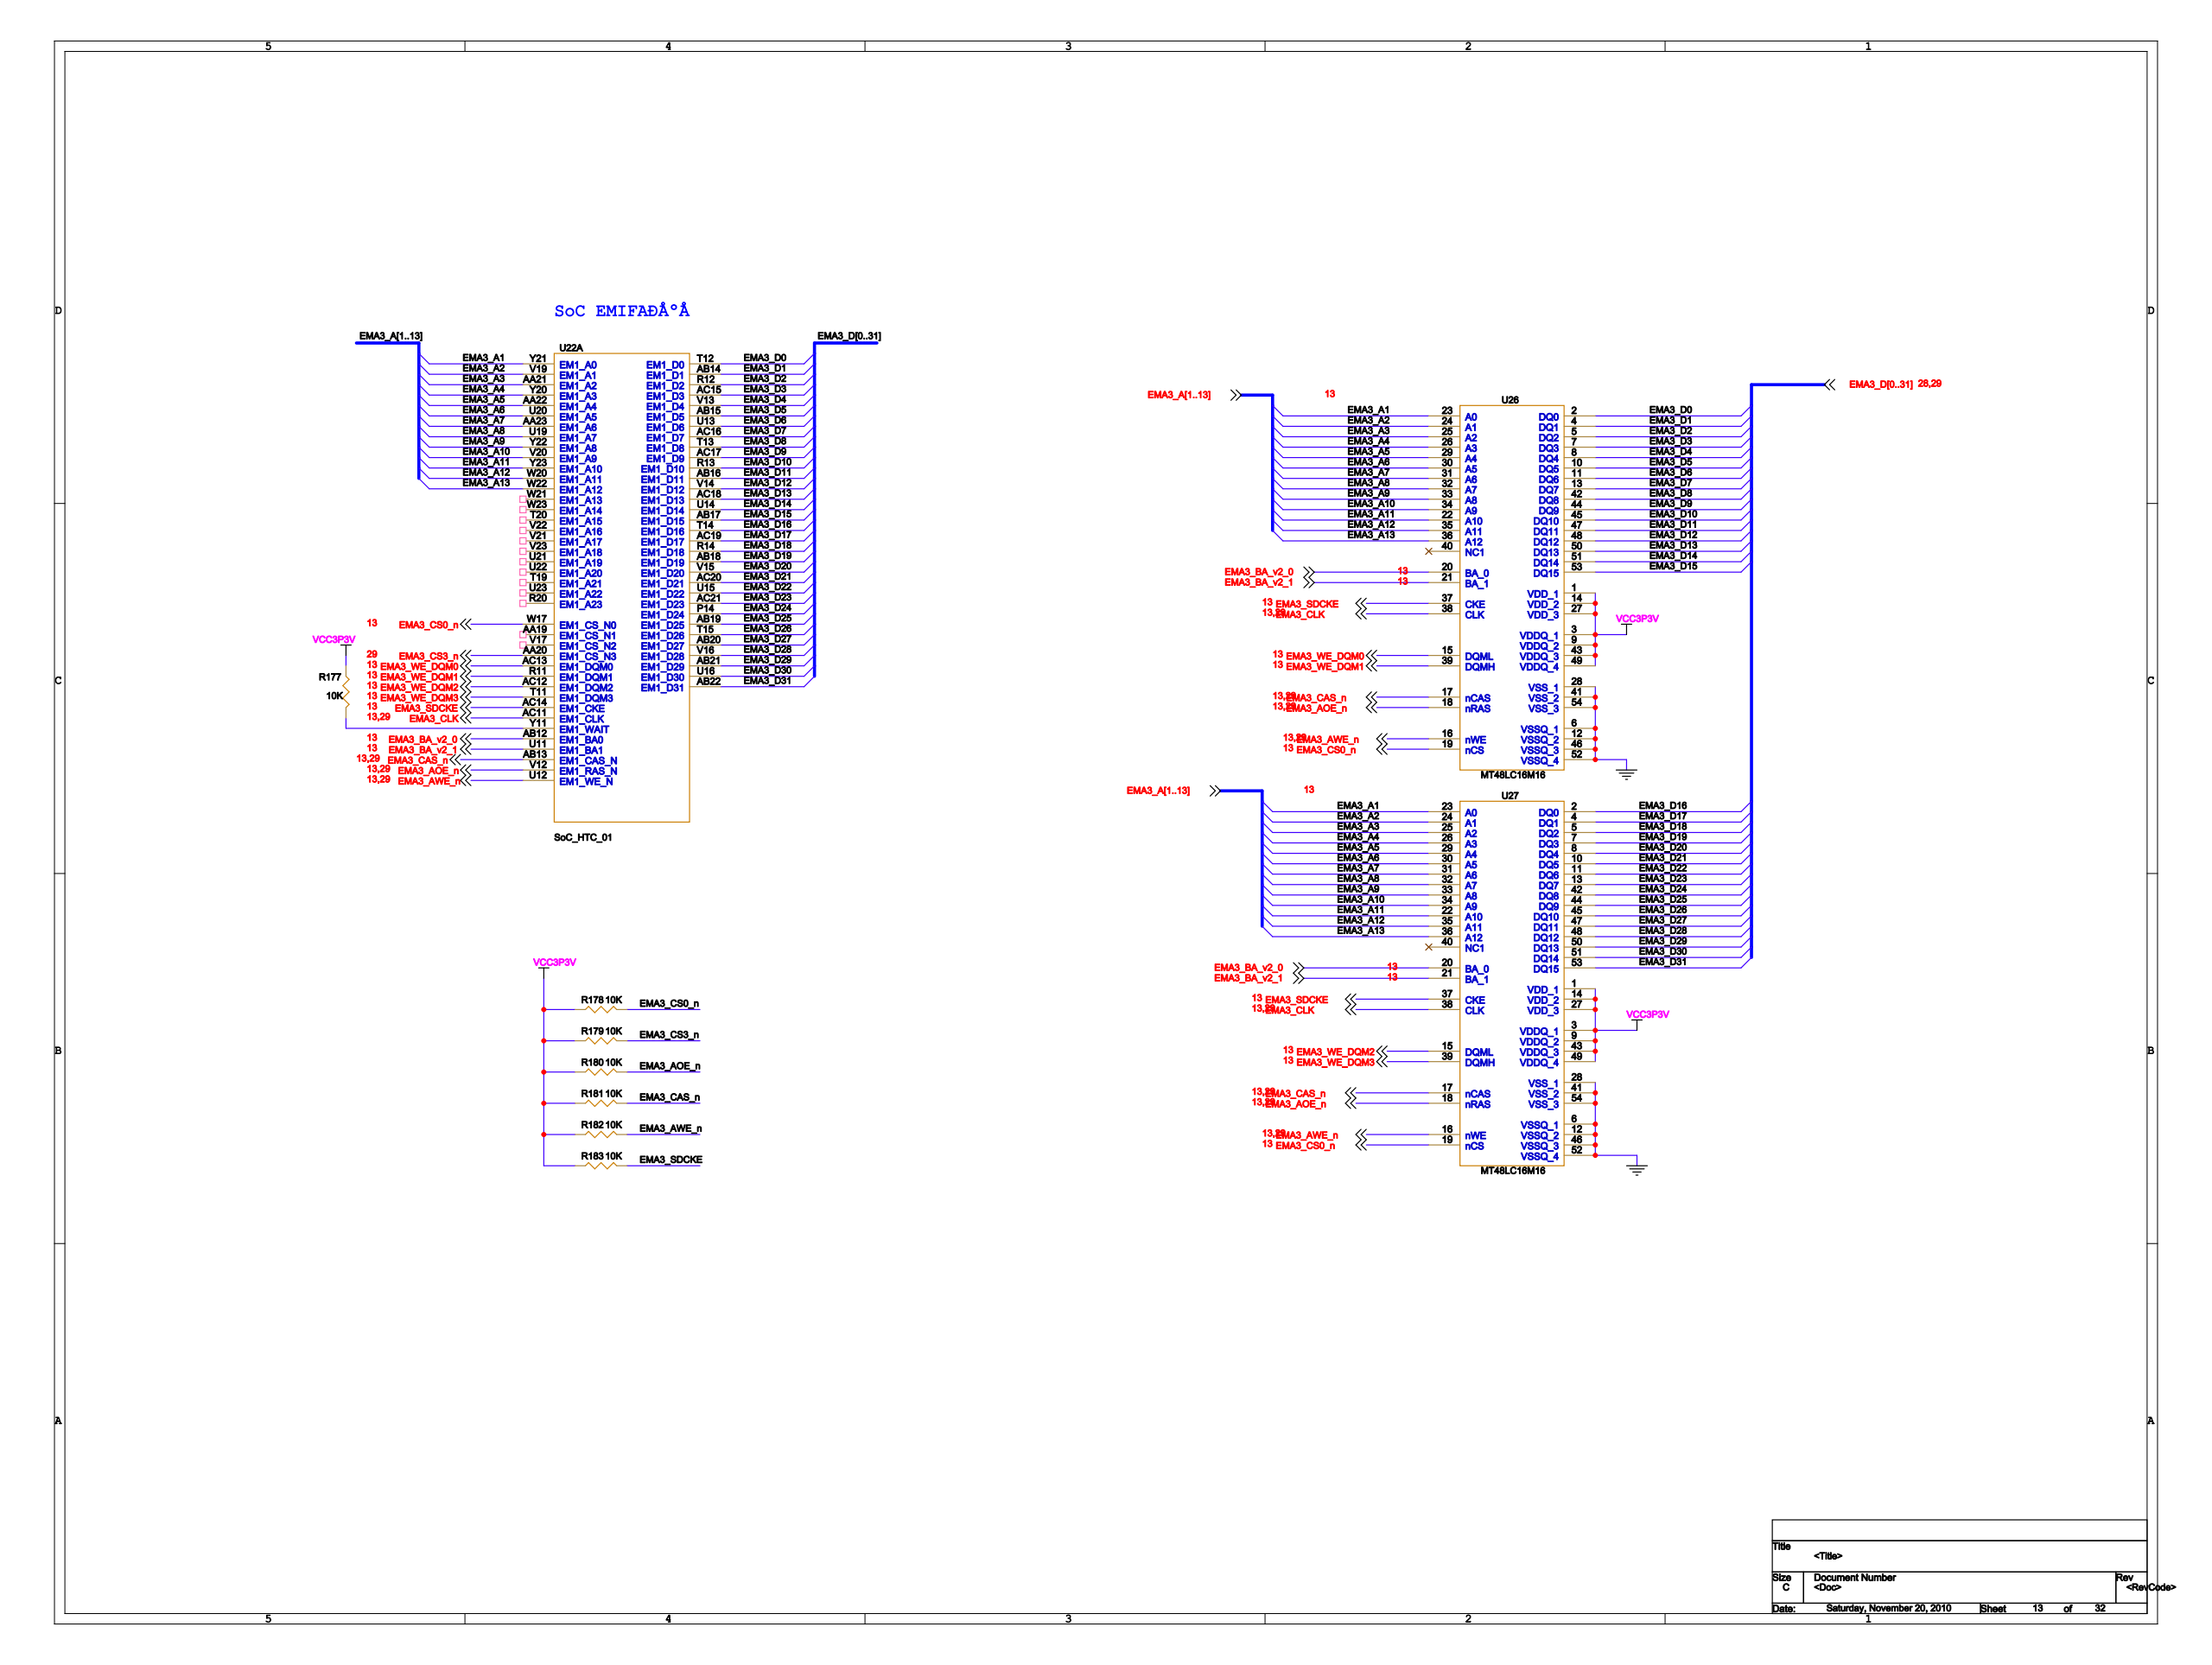Circuit board | Cadence Allegro | 1001 parts | 1318 nets | one sheet of the schematic
Parts on this sheet (reference | value | footprint):
R177 | 10K | 0603
R178 | 10K | 0603
R179 | 10K | 0603
R180 | 10K | 0603
R181 | 10K | 0603
R182 | 10K | 0603
R183 | 10K | 0603
U11 | MT48LC32M16 | TSOP54
U14 | MT48LC16M16 | TSOP54
U15 | MT48LC16M16 | TSOP54
U20 | MT48LC16M16 | TSOP54
U21 | MT48LC16M16 | TSOP54
U22 | SoC_HTC_01 | L529_XIN
U23 | MT48LC32M16 | TSOP54
U26 | MT48LC16M16 | TSOP54
U27 | MT48LC16M16 | TSOP54
Nets of these parts (net: part-pin ...):
EMA3_AWE_N: R182-2 U22-U12 U26-16 U27-16
EMA3_D6: U22-U13 U26-11
EMA3_D0: U22-T12 U26-2
EMA3_D2: U22-R12 U26-5
EMA3_D8: U22-T13 U26-42
EMA3_D10: U22-R13 U26-45
EMA3_D18: U22-R14 U27-5
EMA3_CLK: U22-AC11 U26-38 U27-38
EMA3_D16: U22-T14 U27-2
EMA3_D24: U22-P14 U27-42
EMA3_D22: U22-U15 U27-11
EMA3_D20: U22-V15 U27-8
EMA3_D26: U22-T15 U27-45
EMA3_D30: U22-U16 U27-51
EMA3_D23: U22-AC21 U27-13
EMA3_D31: U22-AB22 U27-53
EMA3_D14: U22-U14 U26-51
EMA3_D12: U22-V14 U26-48
EMA3_D28: U22-V16 U27-48
EMA3_CAS_N: R181-2 U22-AB13 U26-17 U27-17
EMA3_D5: U22-AB15 U26-10
EMA3_D1: U22-AB14 U26-4
EMA3_D3: U22-AC15 U26-7
EMA3_D11: U22-AB16 U26-47
EMA3_D15: U22-AB17 U26-53
EMA3_D7: U22-AC16 U26-13
EMA3_D25: U22-AB19 U27-44
EMA3_D19: U22-AB18 U27-7
EMA3_D9: U22-AC17 U26-44
EMA3_D21: U22-AC20 U27-10
EMA3_D13: U22-AC18 U26-50
EMA3_D27: U22-AB20 U27-47
EMA3_D17: U22-AC19 U27-4
EMA3_CS3_N: R179-2 U22-AA20
EMA3_D29: U22-AB21 U27-50
EMA3_D4: U22-V13 U26-8
EMA3_AOE_N: R180-2 U22-V12 U26-18 U27-18
VCC3P3V: R177-2 R178-1 R179-1 R180-1 R181-1 R182-1 R183-1 U11-1 U11-3 U11-9 U11-14 U11-27 U11-43 U11-49 U14-1 U14-3 U14-9 U14-14 U14-27 U14-43 U14-49 U15-1 U15-3 U15-9 U15-14 U15-27 U15-43 U15-49 U20-1 U20-3 U20-9 U20-14 U20-27 U20-43 U20-49 U21-1 U21-3 U21-9 U21-14 U21-27 U21-43 U21-49 U23-1 U23-3 U23-9 U23-14 U23-27 U23-43 U23-49 U26-1 U26-3 U26-9 U26-14 U26-27 U26-43 U26-49 U27-1 U27-3 U27-9 U27-14 U27-27 U27-43 U27-49
EMA3_A1: U22-Y21 U26-23 U27-23
EMA3_A2: U22-V19 U26-24 U27-24
EMA3_A11: U22-Y23 U26-22 U27-22
EMA3_A12: U22-W20 U26-35 U27-35
EMA3_A13: U22-W22 U26-36 U27-36
EMA3_A3: U22-AA21 U26-25 U27-25
EMA3_A4: U22-Y20 U26-26 U27-26
EMA3_A5: U22-AA22 U26-29 U27-29
EMA3_A6: U22-U20 U26-30 U27-30
EMA3_A7: U22-AA23 U26-31 U27-31
EMA3_A8: U22-U19 U26-32 U27-32
EMA3_A9: U22-Y22 U26-33 U27-33
EMA3_A10: U22-V20 U26-34 U27-34
EMA3_SDCKE: R183-2 U22-AC14 U26-37 U27-37
EMA3_CS0_N: R178-2 U22-W17 U26-19 U27-19
EMA3_WE_DQM0: U22-AC13 U26-15
EMA3_WE_DQM1: U22-R11 U26-39
EMA3_WE_DQM2: U22-AC12 U27-15
EMA3_WE_DQM3: U22-T11 U27-39
N16816470: R177-1 U22-Y11